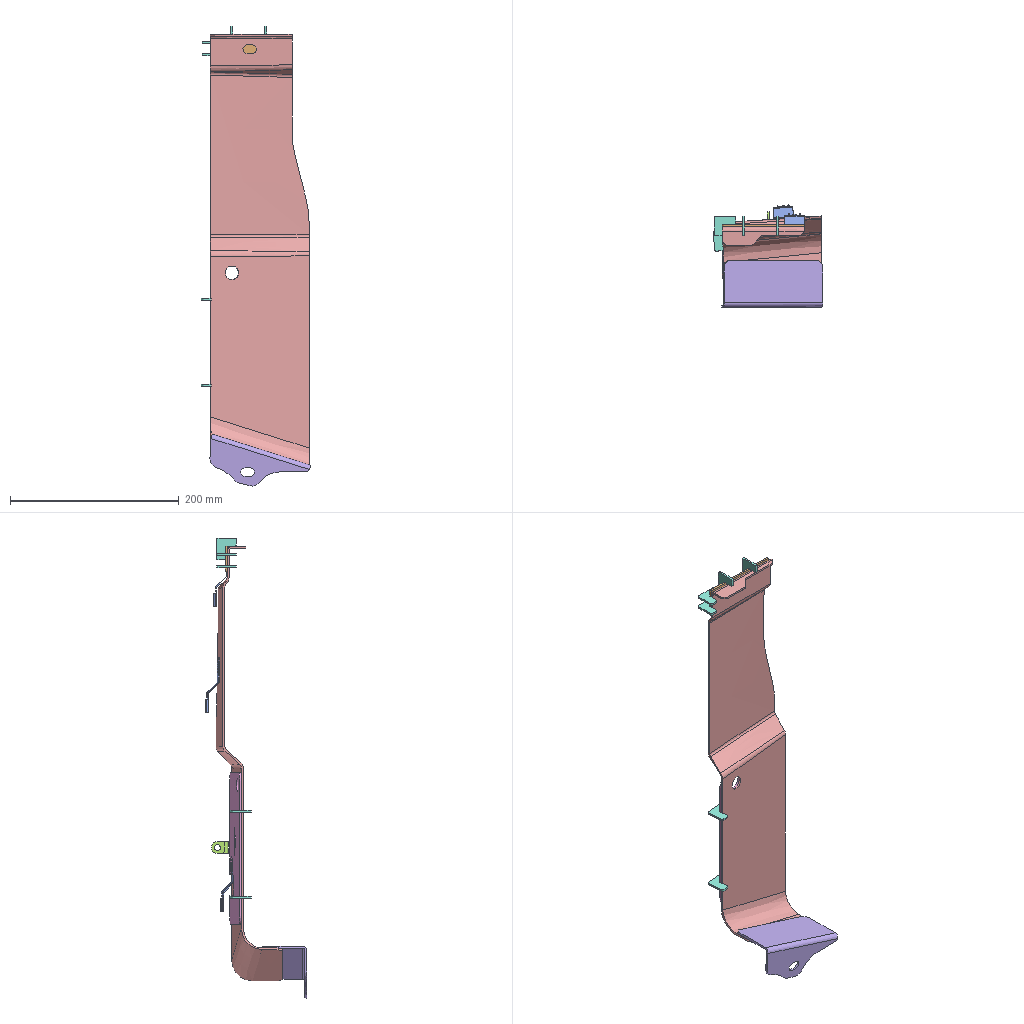Assembly | SolidWorks | 7 different items | 14 placed | box 130 x 121 x 545 mm
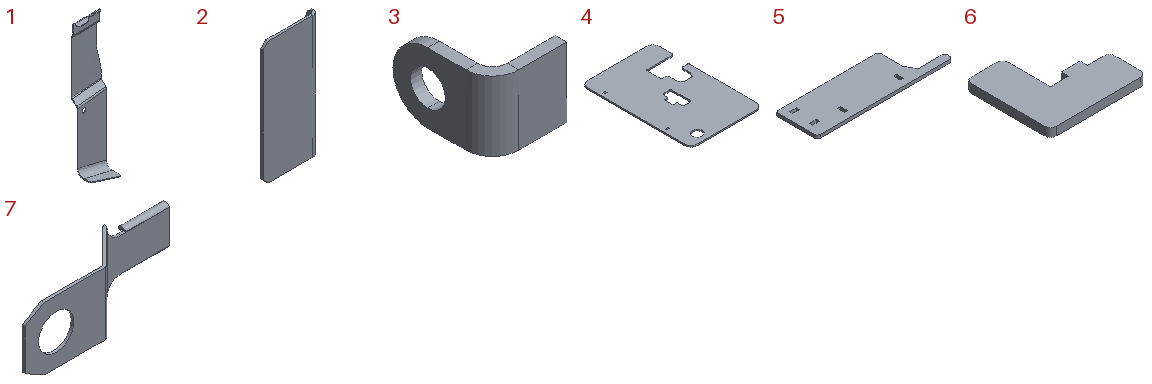Parts list (item | quantity | size | volume | features):
1 | x1 | 116.807 x 78.32 x 514.503 mm | 142015 mm3 | features BaseBody 1
2 | x1 | 55 x 45.365 x 122.5 mm | 22297 mm3 | features Chamfer 1, Fillet 1, FlatPattern 1, ICE 1, SMBaseFlange 1, SheetMetal 1
3 | x1 | 15 x 20 x 14 mm | 858.7 mm3 | features Fillet 1, FlatPattern 1, ICE 1, SMBaseFlange 1, SheetMetal 1
4 | x1 | 117.378 x 180 x 2.3 mm | 42940 mm3 | features FlatPattern 1, SMBaseFlange 1, SheetMetal 1
5 | x1 | 96.8 x 30.001 x 2.3 mm | 5301 mm3 | features FlatPattern 1, SMBaseFlange 1, SheetMetal 1
6 | x6 | 26 x 23 x 2.3 mm | 914.447 mm3 | features FlatPattern 1, SMBaseFlange 1, SheetMetal 1
7 | x3 | 65.7 x 15.573 x 23.06 mm | 1342 mm3 | features BaseBody 1
Mates (type | each side: item.copy, entity, surface, feature):
Coincident | 5.1 face plane Base-Flange1 | 6.1 face plane Base-Flange1 | 3 times
Coincident | 5.1 face plane Base-Flange1 | 6.2 face plane Base-Flange1 | 3 times
Coincident | 5.1 face plane Base-Flange1 | 6.3 face plane Base-Flange1 | 3 times
Coincident | 5.1 face plane Base-Flange1 | 6.4 face plane Base-Flange1 | 3 times
Tangent | 1.1 face surface:4006 Input1 | 2.1 face plane Base-Flange1